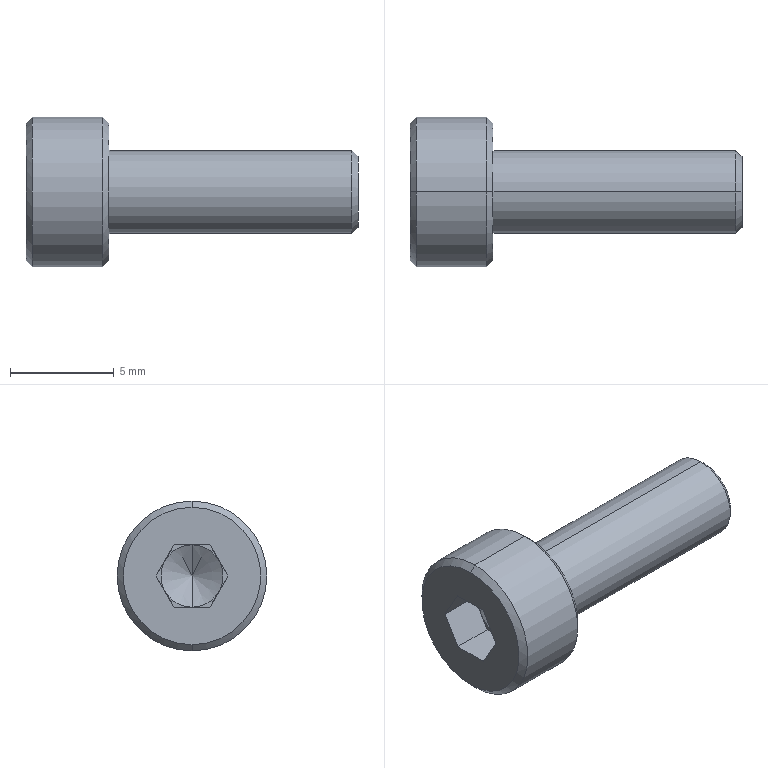Part | STEP file | Hex socket screw Dongming full thread M4-12 A2-70-1 | 1 solid | 27 faces | box 16 x 7.22 x 7.22 mm | volume 294.412 mm3 | plane 15 | cone 8 | cylinder 4 | commonest cylinder face diameters 4 x2 7.22 x2
STEP:
#1=CARTESIAN_POINT('',(16.,0.,-1.7));
#2=VERTEX_POINT('',#1);
#3=CARTESIAN_POINT('',(16.,0.,1.7));
#4=VERTEX_POINT('',#3);
#5=CARTESIAN_POINT('',(16.,0.,0.));
#6=DIRECTION('',(1.,0.,0.));
#7=DIRECTION('',(0.,0.,-1.));
#8=AXIS2_PLACEMENT_3D('',#5,#6,#7);
#9=CIRCLE('',#8,1.7);
#10=EDGE_CURVE('',#2,#4,#9,.T.);
#11=ORIENTED_EDGE('',*,*,#10,.F.);
#12=CARTESIAN_POINT('',(15.7,0.,-2.));
#13=VERTEX_POINT('',#12);
#14=CARTESIAN_POINT('',(16.,0.,-1.7));
#15=DIRECTION('',(-0.7071,0.,-0.7071));
#16=VECTOR('',#15,1000.);
#17=LINE('',#14,#16);
#18=EDGE_CURVE('',#2,#13,#17,.T.);
#19=ORIENTED_EDGE('',*,*,#18,.T.);
#20=CARTESIAN_POINT('',(15.7,0.,2.));
#21=VERTEX_POINT('',#20);
#22=CARTESIAN_POINT('',(15.7,0.,0.));
#23=DIRECTION('',(-1.,0.,0.));
#24=DIRECTION('',(0.,0.,-1.));
#25=AXIS2_PLACEMENT_3D('',#22,#23,#24);
#26=CIRCLE('',#25,2.);
#27=EDGE_CURVE('',#21,#13,#26,.T.);
#28=ORIENTED_EDGE('',*,*,#27,.F.);
#29=CARTESIAN_POINT('',(16.,0.,1.7));
#30=DIRECTION('',(-0.7071,0.,0.7071));
#31=VECTOR('',#30,1000.);
#32=LINE('',#29,#31);
#33=EDGE_CURVE('',#4,#21,#32,.T.);
#34=ORIENTED_EDGE('',*,*,#33,.F.);
#35=EDGE_LOOP('',(#11,#19,#28,#34));
#36=FACE_OUTER_BOUND('',#35,.T.);
#37=CARTESIAN_POINT('',(16.,0.,0.));
#38=DIRECTION('',(-1.,0.,0.));
#39=DIRECTION('',(0.,0.,1.));
#40=AXIS2_PLACEMENT_3D('',#37,#38,#39);
#41=CONICAL_SURFACE('',#40,1.7,0.7854);
#42=ADVANCED_FACE('',(#36),#41,.T.);
#43=CARTESIAN_POINT('',(4.,0.,-3.31));
#44=VERTEX_POINT('',#43);
#45=CARTESIAN_POINT('',(4.,0.,3.31));
#46=VERTEX_POINT('',#45);
#47=CARTESIAN_POINT('',(4.,0.,0.));
#48=DIRECTION('',(1.,0.,0.));
#49=DIRECTION('',(0.,0.,-1.));
#50=AXIS2_PLACEMENT_3D('',#47,#48,#49);
#51=CIRCLE('',#50,3.31);
#52=EDGE_CURVE('',#44,#46,#51,.T.);
#53=ORIENTED_EDGE('',*,*,#52,.F.);
#54=CARTESIAN_POINT('',(3.7,0.,-3.61));
#55=VERTEX_POINT('',#54);
#56=CARTESIAN_POINT('',(4.,0.,-3.31));
#57=DIRECTION('',(-0.7071,0.,-0.7071));
#58=VECTOR('',#57,1000.);
#59=LINE('',#56,#58);
#60=EDGE_CURVE('',#44,#55,#59,.T.);
#61=ORIENTED_EDGE('',*,*,#60,.T.);
#62=CARTESIAN_POINT('',(3.7,0.,3.61));
#63=VERTEX_POINT('',#62);
#64=CARTESIAN_POINT('',(3.7,0.,0.));
#65=DIRECTION('',(-1.,0.,0.));
#66=DIRECTION('',(0.,0.,-1.));
#67=AXIS2_PLACEMENT_3D('',#64,#65,#66);
#68=CIRCLE('',#67,3.61);
#69=EDGE_CURVE('',#63,#55,#68,.T.);
#70=ORIENTED_EDGE('',*,*,#69,.F.);
#71=CARTESIAN_POINT('',(4.,0.,3.31));
#72=DIRECTION('',(-0.7071,0.,0.7071));
#73=VECTOR('',#72,1000.);
#74=LINE('',#71,#73);
#75=EDGE_CURVE('',#46,#63,#74,.T.);
#76=ORIENTED_EDGE('',*,*,#75,.F.);
#77=EDGE_LOOP('',(#53,#61,#70,#76));
#78=FACE_OUTER_BOUND('',#77,.T.);
#79=CARTESIAN_POINT('',(4.,0.,0.));
#80=DIRECTION('',(-1.,0.,0.));
#81=DIRECTION('',(0.,0.,1.));
#82=AXIS2_PLACEMENT_3D('',#79,#80,#81);
#83=CONICAL_SURFACE('',#82,3.31,0.7854);
#84=ADVANCED_FACE('',(#78),#83,.T.);
#85=CARTESIAN_POINT('',(0.,0.,3.31));
#86=VERTEX_POINT('',#85);
#87=CARTESIAN_POINT('',(0.,0.,-3.31));
#88=VERTEX_POINT('',#87);
#89=CARTESIAN_POINT('',(0.,0.,0.));
#90=DIRECTION('',(-1.,0.,0.));
#91=DIRECTION('',(0.,0.,-1.));
#92=AXIS2_PLACEMENT_3D('',#89,#90,#91);
#93=CIRCLE('',#92,3.31);
#94=EDGE_CURVE('',#86,#88,#93,.T.);
#95=ORIENTED_EDGE('',*,*,#94,.F.);
#96=CARTESIAN_POINT('',(0.3,0.,3.61));
#97=VERTEX_POINT('',#96);
#98=CARTESIAN_POINT('',(0.3,0.,3.61));
#99=DIRECTION('',(0.7071,0.,0.7071));
#100=VECTOR('',#99,1000.);
#101=LINE('',#98,#100);
#102=EDGE_CURVE('',#86,#97,#101,.T.);
#103=ORIENTED_EDGE('',*,*,#102,.T.);
#104=CARTESIAN_POINT('',(0.3,0.,-3.61));
#105=VERTEX_POINT('',#104);
#106=CARTESIAN_POINT('',(0.3,0.,0.));
#107=DIRECTION('',(1.,0.,0.));
#108=DIRECTION('',(0.,0.,-1.));
#109=AXIS2_PLACEMENT_3D('',#106,#107,#108);
#110=CIRCLE('',#109,3.61);
#111=EDGE_CURVE('',#105,#97,#110,.T.);
#112=ORIENTED_EDGE('',*,*,#111,.F.);
#113=CARTESIAN_POINT('',(0.3,0.,-3.61));
#114=DIRECTION('',(0.7071,0.,-0.7071));
#115=VECTOR('',#114,1000.);
#116=LINE('',#113,#115);
#117=EDGE_CURVE('',#88,#105,#116,.T.);
#118=ORIENTED_EDGE('',*,*,#117,.F.);
#119=EDGE_LOOP('',(#95,#103,#112,#118));
#120=FACE_OUTER_BOUND('',#119,.T.);
#121=CARTESIAN_POINT('',(0.3,0.,0.));
#122=DIRECTION('',(1.,0.,0.));
#123=DIRECTION('',(0.,0.,-1.));
#124=AXIS2_PLACEMENT_3D('',#121,#122,#123);
#125=CONICAL_SURFACE('',#124,3.61,0.7854);
#126=ADVANCED_FACE('',(#120),#125,.T.);
#127=CARTESIAN_POINT('',(2.866,0.,0.));
#128=VERTEX_POINT('',#127);
#129=CARTESIAN_POINT('',(2.,0.,1.5));
#130=VERTEX_POINT('',#129);
#131=CARTESIAN_POINT('',(2.866,0.,0.));
#132=DIRECTION('',(-0.5,0.,0.866));
#133=VECTOR('',#132,1000.);
#134=LINE('',#131,#133);
#135=EDGE_CURVE('',#128,#130,#134,.T.);
#136=ORIENTED_EDGE('',*,*,#135,.F.);
#137=CARTESIAN_POINT('',(2.,0.,-1.5));
#138=VERTEX_POINT('',#137);
#139=CARTESIAN_POINT('',(2.866,0.,0.));
#140=DIRECTION('',(-0.5,0.,-0.866));
#141=VECTOR('',#140,1000.);
#142=LINE('',#139,#141);
#143=EDGE_CURVE('',#128,#138,#142,.T.);
#144=ORIENTED_EDGE('',*,*,#143,.T.);
#145=CARTESIAN_POINT('',(2.,-1.299,-0.75));
#146=VERTEX_POINT('',#145);
#147=CARTESIAN_POINT('',(2.,0.,0.));
#148=DIRECTION('',(-1.,0.,0.));
#149=DIRECTION('',(0.,0.,1.));
#150=AXIS2_PLACEMENT_3D('',#147,#148,#149);
#151=CIRCLE('',#150,1.5);
#152=EDGE_CURVE('',#138,#146,#151,.T.);
#153=ORIENTED_EDGE('',*,*,#152,.T.);
#154=CARTESIAN_POINT('',(2.,-1.299,0.75));
#155=VERTEX_POINT('',#154);
#156=CARTESIAN_POINT('',(2.,0.,0.));
#157=DIRECTION('',(-1.,0.,0.));
#158=DIRECTION('',(0.,0.,1.));
#159=AXIS2_PLACEMENT_3D('',#156,#157,#158);
#160=CIRCLE('',#159,1.5);
#161=EDGE_CURVE('',#146,#155,#160,.T.);
#162=ORIENTED_EDGE('',*,*,#161,.T.);
#163=CARTESIAN_POINT('',(2.,0.,0.));
#164=DIRECTION('',(-1.,0.,0.));
#165=DIRECTION('',(0.,0.,1.));
#166=AXIS2_PLACEMENT_3D('',#163,#164,#165);
#167=CIRCLE('',#166,1.5);
#168=EDGE_CURVE('',#155,#130,#167,.T.);
#169=ORIENTED_EDGE('',*,*,#168,.T.);
#170=EDGE_LOOP('',(#136,#144,#153,#162,#169));
#171=FACE_OUTER_BOUND('',#170,.T.);
#172=CARTESIAN_POINT('',(-997.134,0.,0.));
#173=DIRECTION('',(-1.,0.,0.));
#174=DIRECTION('',(0.,0.,1.));
#175=AXIS2_PLACEMENT_3D('',#172,#173,#174);
#176=CONICAL_SURFACE('',#175,1732.051,1.047);
#177=ADVANCED_FACE('',(#171),#176,.F.);
#178=ORIENTED_EDGE('',*,*,#27,.T.);
#179=CARTESIAN_POINT('',(4.,0.,-2.));
#180=VERTEX_POINT('',#179);
#181=CARTESIAN_POINT('',(16.,0.,-2.));
#182=DIRECTION('',(-1.,0.,0.));
#183=VECTOR('',#182,1000.);
#184=LINE('',#181,#183);
#185=EDGE_CURVE('',#13,#180,#184,.T.);
#186=ORIENTED_EDGE('',*,*,#185,.T.);
#187=CARTESIAN_POINT('',(4.,0.,2.));
#188=VERTEX_POINT('',#187);
#189=CARTESIAN_POINT('',(4.,0.,0.));
#190=DIRECTION('',(1.,0.,0.));
#191=DIRECTION('',(0.,0.,-1.));
#192=AXIS2_PLACEMENT_3D('',#189,#190,#191);
#193=CIRCLE('',#192,2.);
#194=EDGE_CURVE('',#180,#188,#193,.T.);
#195=ORIENTED_EDGE('',*,*,#194,.T.);
#196=CARTESIAN_POINT('',(16.,0.,2.));
#197=DIRECTION('',(-1.,0.,0.));
#198=VECTOR('',#197,1000.);
#199=LINE('',#196,#198);
#200=EDGE_CURVE('',#21,#188,#199,.T.);
#201=ORIENTED_EDGE('',*,*,#200,.F.);
#202=EDGE_LOOP('',(#178,#186,#195,#201));
#203=FACE_OUTER_BOUND('',#202,.T.);
#204=CARTESIAN_POINT('',(16.,0.,0.));
#205=DIRECTION('',(-1.,0.,0.));
#206=DIRECTION('',(0.,0.,1.));
#207=AXIS2_PLACEMENT_3D('',#204,#205,#206);
#208=CYLINDRICAL_SURFACE('',#207,2.);
#209=ADVANCED_FACE('',(#203),#208,.T.);
#210=ORIENTED_EDGE('',*,*,#69,.T.);
#211=CARTESIAN_POINT('',(4.,0.,-3.61));
#212=DIRECTION('',(-1.,0.,0.));
#213=VECTOR('',#212,1000.);
#214=LINE('',#211,#213);
#215=EDGE_CURVE('',#55,#105,#214,.T.);
#216=ORIENTED_EDGE('',*,*,#215,.T.);
#217=ORIENTED_EDGE('',*,*,#111,.T.);
#218=CARTESIAN_POINT('',(4.,0.,3.61));
#219=DIRECTION('',(-1.,0.,0.));
#220=VECTOR('',#219,1000.);
#221=LINE('',#218,#220);
#222=EDGE_CURVE('',#63,#97,#221,.T.);
#223=ORIENTED_EDGE('',*,*,#222,.F.);
#224=EDGE_LOOP('',(#210,#216,#217,#223));
#225=FACE_OUTER_BOUND('',#224,.T.);
#226=CARTESIAN_POINT('',(4.,0.,0.));
#227=DIRECTION('',(-1.,0.,0.));
#228=DIRECTION('',(0.,0.,1.));
#229=AXIS2_PLACEMENT_3D('',#226,#227,#228);
#230=CYLINDRICAL_SURFACE('',#229,3.61);
#231=ADVANCED_FACE('',(#225),#230,.T.);
#232=CARTESIAN_POINT('',(2.,1.299,0.75));
#233=VERTEX_POINT('',#232);
#234=CARTESIAN_POINT('',(2.,0.,0.));
#235=DIRECTION('',(-1.,0.,0.));
#236=DIRECTION('',(0.,0.,1.));
#237=AXIS2_PLACEMENT_3D('',#234,#235,#236);
#238=CIRCLE('',#237,1.5);
#239=EDGE_CURVE('',#130,#233,#238,.T.);
#240=ORIENTED_EDGE('',*,*,#239,.F.);
#241=CARTESIAN_POINT('',(2.,0.866,1.5));
#242=VERTEX_POINT('',#241);
#243=CARTESIAN_POINT('',(2.,-0.866,1.5));
#244=DIRECTION('',(0.,1.,0.));
#245=VECTOR('',#244,1000.);
#246=LINE('',#243,#245);
#247=EDGE_CURVE('',#130,#242,#246,.T.);
#248=ORIENTED_EDGE('',*,*,#247,.T.);
#249=CARTESIAN_POINT('',(2.,0.866,1.5));
#250=DIRECTION('',(0.,0.5,-0.866));
#251=VECTOR('',#250,1000.);
#252=LINE('',#249,#251);
#253=EDGE_CURVE('',#242,#233,#252,.T.);
#254=ORIENTED_EDGE('',*,*,#253,.T.);
#255=EDGE_LOOP('',(#240,#248,#254));
#256=FACE_OUTER_BOUND('',#255,.T.);
#257=CARTESIAN_POINT('',(2.,0.,0.));
#258=DIRECTION('',(-1.,0.,0.));
#259=DIRECTION('',(0.,0.,1.));
#260=AXIS2_PLACEMENT_3D('',#257,#258,#259);
#261=PLANE('',#260);
#262=ADVANCED_FACE('',(#256),#261,.T.);
#263=CARTESIAN_POINT('',(2.,1.299,-0.75));
#264=VERTEX_POINT('',#263);
#265=CARTESIAN_POINT('',(2.,0.,0.));
#266=DIRECTION('',(-1.,0.,0.));
#267=DIRECTION('',(0.,0.,1.));
#268=AXIS2_PLACEMENT_3D('',#265,#266,#267);
#269=CIRCLE('',#268,1.5);
#270=EDGE_CURVE('',#233,#264,#269,.T.);
#271=ORIENTED_EDGE('',*,*,#270,.F.);
#272=CARTESIAN_POINT('',(2.,1.732,0.));
#273=VERTEX_POINT('',#272);
#274=CARTESIAN_POINT('',(2.,0.866,1.5));
#275=DIRECTION('',(0.,0.5,-0.866));
#276=VECTOR('',#275,1000.);
#277=LINE('',#274,#276);
#278=EDGE_CURVE('',#233,#273,#277,.T.);
#279=ORIENTED_EDGE('',*,*,#278,.T.);
#280=CARTESIAN_POINT('',(2.,1.732,0.));
#281=DIRECTION('',(0.,-0.5,-0.866));
#282=VECTOR('',#281,1000.);
#283=LINE('',#280,#282);
#284=EDGE_CURVE('',#273,#264,#283,.T.);
#285=ORIENTED_EDGE('',*,*,#284,.T.);
#286=EDGE_LOOP('',(#271,#279,#285));
#287=FACE_OUTER_BOUND('',#286,.T.);
#288=CARTESIAN_POINT('',(2.,0.,0.));
#289=DIRECTION('',(-1.,0.,0.));
#290=DIRECTION('',(0.,0.,1.));
#291=AXIS2_PLACEMENT_3D('',#288,#289,#290);
#292=PLANE('',#291);
#293=ADVANCED_FACE('',(#287),#292,.T.);
#294=CARTESIAN_POINT('',(2.,0.,0.));
#295=DIRECTION('',(-1.,0.,0.));
#296=DIRECTION('',(0.,0.,1.));
#297=AXIS2_PLACEMENT_3D('',#294,#295,#296);
#298=CIRCLE('',#297,1.5);
#299=EDGE_CURVE('',#264,#138,#298,.T.);
#300=ORIENTED_EDGE('',*,*,#299,.F.);
#301=CARTESIAN_POINT('',(2.,0.866,-1.5));
#302=VERTEX_POINT('',#301);
#303=CARTESIAN_POINT('',(2.,1.732,0.));
#304=DIRECTION('',(0.,-0.5,-0.866));
#305=VECTOR('',#304,1000.);
#306=LINE('',#303,#305);
#307=EDGE_CURVE('',#264,#302,#306,.T.);
#308=ORIENTED_EDGE('',*,*,#307,.T.);
#309=CARTESIAN_POINT('',(2.,0.866,-1.5));
#310=DIRECTION('',(0.,-1.,0.));
#311=VECTOR('',#310,1000.);
#312=LINE('',#309,#311);
#313=EDGE_CURVE('',#302,#138,#312,.T.);
#314=ORIENTED_EDGE('',*,*,#313,.T.);
#315=EDGE_LOOP('',(#300,#308,#314));
#316=FACE_OUTER_BOUND('',#315,.T.);
#317=CARTESIAN_POINT('',(2.,0.,0.));
#318=DIRECTION('',(-1.,0.,0.));
#319=DIRECTION('',(0.,0.,1.));
#320=AXIS2_PLACEMENT_3D('',#317,#318,#319);
#321=PLANE('',#320);
#322=ADVANCED_FACE('',(#316),#321,.T.);
#323=ORIENTED_EDGE('',*,*,#152,.F.);
#324=CARTESIAN_POINT('',(2.,-0.866,-1.5));
#325=VERTEX_POINT('',#324);
#326=CARTESIAN_POINT('',(2.,0.866,-1.5));
#327=DIRECTION('',(0.,-1.,0.));
#328=VECTOR('',#327,1000.);
#329=LINE('',#326,#328);
#330=EDGE_CURVE('',#138,#325,#329,.T.);
#331=ORIENTED_EDGE('',*,*,#330,.T.);
#332=CARTESIAN_POINT('',(2.,-0.866,-1.5));
#333=DIRECTION('',(0.,-0.5,0.866));
#334=VECTOR('',#333,1000.);
#335=LINE('',#332,#334);
#336=EDGE_CURVE('',#325,#146,#335,.T.);
#337=ORIENTED_EDGE('',*,*,#336,.T.);
#338=EDGE_LOOP('',(#323,#331,#337));
#339=FACE_OUTER_BOUND('',#338,.T.);
#340=CARTESIAN_POINT('',(2.,0.,0.));
#341=DIRECTION('',(-1.,0.,0.));
#342=DIRECTION('',(0.,0.,1.));
#343=AXIS2_PLACEMENT_3D('',#340,#341,#342);
#344=PLANE('',#343);
#345=ADVANCED_FACE('',(#339),#344,.T.);
#346=ORIENTED_EDGE('',*,*,#161,.F.);
#347=CARTESIAN_POINT('',(2.,-1.732,0.));
#348=VERTEX_POINT('',#347);
#349=CARTESIAN_POINT('',(2.,-0.866,-1.5));
#350=DIRECTION('',(0.,-0.5,0.866));
#351=VECTOR('',#350,1000.);
#352=LINE('',#349,#351);
#353=EDGE_CURVE('',#146,#348,#352,.T.);
#354=ORIENTED_EDGE('',*,*,#353,.T.);
#355=CARTESIAN_POINT('',(2.,-1.732,0.));
#356=DIRECTION('',(0.,0.5,0.866));
#357=VECTOR('',#356,1000.);
#358=LINE('',#355,#357);
#359=EDGE_CURVE('',#348,#155,#358,.T.);
#360=ORIENTED_EDGE('',*,*,#359,.T.);
#361=EDGE_LOOP('',(#346,#354,#360));
#362=FACE_OUTER_BOUND('',#361,.T.);
#363=CARTESIAN_POINT('',(2.,0.,0.));
#364=DIRECTION('',(-1.,0.,0.));
#365=DIRECTION('',(0.,0.,1.));
#366=AXIS2_PLACEMENT_3D('',#363,#364,#365);
#367=PLANE('',#366);
#368=ADVANCED_FACE('',(#362),#367,.T.);
#369=ORIENTED_EDGE('',*,*,#215,.F.);
#370=CARTESIAN_POINT('',(3.7,0.,0.));
#371=DIRECTION('',(-1.,0.,0.));
#372=DIRECTION('',(0.,0.,-1.));
#373=AXIS2_PLACEMENT_3D('',#370,#371,#372);
#374=CIRCLE('',#373,3.61);
#375=EDGE_CURVE('',#55,#63,#374,.T.);
#376=ORIENTED_EDGE('',*,*,#375,.T.);
#377=ORIENTED_EDGE('',*,*,#222,.T.);
#378=CARTESIAN_POINT('',(0.3,0.,0.));
#379=DIRECTION('',(1.,0.,0.));
#380=DIRECTION('',(0.,0.,-1.));
#381=AXIS2_PLACEMENT_3D('',#378,#379,#380);
#382=CIRCLE('',#381,3.61);
#383=EDGE_CURVE('',#97,#105,#382,.T.);
#384=ORIENTED_EDGE('',*,*,#383,.T.);
#385=EDGE_LOOP('',(#369,#376,#377,#384));
#386=FACE_OUTER_BOUND('',#385,.T.);
#387=CARTESIAN_POINT('',(4.,0.,0.));
#388=DIRECTION('',(-1.,0.,0.));
#389=DIRECTION('',(0.,0.,1.));
#390=AXIS2_PLACEMENT_3D('',#387,#388,#389);
#391=CYLINDRICAL_SURFACE('',#390,3.61);
#392=ADVANCED_FACE('',(#386),#391,.T.);
#393=CARTESIAN_POINT('',(4.,0.,0.));
#394=DIRECTION('',(1.,0.,0.));
#395=DIRECTION('',(0.,0.,-1.));
#396=AXIS2_PLACEMENT_3D('',#393,#394,#395);
#397=CIRCLE('',#396,3.31);
#398=EDGE_CURVE('',#46,#44,#397,.T.);
#399=ORIENTED_EDGE('',*,*,#398,.T.);
#400=ORIENTED_EDGE('',*,*,#52,.T.);
#401=EDGE_LOOP('',(#399,#400));
#402=FACE_OUTER_BOUND('',#401,.T.);
#403=CARTESIAN_POINT('',(4.,0.,0.));
#404=DIRECTION('',(1.,0.,0.));
#405=DIRECTION('',(0.,0.,-1.));
#406=AXIS2_PLACEMENT_3D('',#403,#404,#405);
#407=CIRCLE('',#406,2.);
#408=EDGE_CURVE('',#188,#180,#407,.T.);
#409=ORIENTED_EDGE('',*,*,#408,.F.);
#410=ORIENTED_EDGE('',*,*,#194,.F.);
#411=EDGE_LOOP('',(#409,#410));
#412=FACE_BOUND('',#411,.T.);
#413=CARTESIAN_POINT('',(4.,0.,0.));
#414=DIRECTION('',(1.,0.,0.));
#415=DIRECTION('',(0.,0.,-1.));
#416=AXIS2_PLACEMENT_3D('',#413,#414,#415);
#417=PLANE('',#416);
#418=ADVANCED_FACE('',(#402,#412),#417,.T.);
#419=CARTESIAN_POINT('',(0.,0.,0.));
#420=DIRECTION('',(-1.,0.,0.));
#421=DIRECTION('',(0.,0.,-1.));
#422=AXIS2_PLACEMENT_3D('',#419,#420,#421);
#423=CIRCLE('',#422,3.31);
#424=EDGE_CURVE('',#88,#86,#423,.T.);
#425=ORIENTED_EDGE('',*,*,#424,.T.);
#426=ORIENTED_EDGE('',*,*,#94,.T.);
#427=EDGE_LOOP('',(#425,#426));
#428=FACE_OUTER_BOUND('',#427,.T.);
#429=CARTESIAN_POINT('',(0.,1.732,0.));
#430=VERTEX_POINT('',#429);
#431=CARTESIAN_POINT('',(0.,0.866,-1.5));
#432=VERTEX_POINT('',#431);
#433=CARTESIAN_POINT('',(0.,1.732,0.));
#434=DIRECTION('',(0.,-0.5,-0.866));
#435=VECTOR('',#434,1000.);
#436=LINE('',#433,#435);
#437=EDGE_CURVE('',#430,#432,#436,.T.);
#438=ORIENTED_EDGE('',*,*,#437,.F.);
#439=CARTESIAN_POINT('',(0.,0.866,1.5));
#440=VERTEX_POINT('',#439);
#441=CARTESIAN_POINT('',(0.,0.866,1.5));
#442=DIRECTION('',(0.,0.5,-0.866));
#443=VECTOR('',#442,1000.);
#444=LINE('',#441,#443);
#445=EDGE_CURVE('',#440,#430,#444,.T.);
#446=ORIENTED_EDGE('',*,*,#445,.F.);
#447=CARTESIAN_POINT('',(0.,-0.866,1.5));
#448=VERTEX_POINT('',#447);
#449=CARTESIAN_POINT('',(0.,-0.866,1.5));
#450=DIRECTION('',(0.,1.,0.));
#451=VECTOR('',#450,1000.);
#452=LINE('',#449,#451);
#453=EDGE_CURVE('',#448,#440,#452,.T.);
#454=ORIENTED_EDGE('',*,*,#453,.F.);
#455=CARTESIAN_POINT('',(0.,-1.732,0.));
#456=VERTEX_POINT('',#455);
#457=CARTESIAN_POINT('',(0.,-1.732,0.));
#458=DIRECTION('',(0.,0.5,0.866));
#459=VECTOR('',#458,1000.);
#460=LINE('',#457,#459);
#461=EDGE_CURVE('',#456,#448,#460,.T.);
#462=ORIENTED_EDGE('',*,*,#461,.F.);
#463=CARTESIAN_POINT('',(0.,-0.866,-1.5));
#464=VERTEX_POINT('',#463);
#465=CARTESIAN_POINT('',(0.,-0.866,-1.5));
#466=DIRECTION('',(0.,-0.5,0.866));
#467=VECTOR('',#466,1000.);
#468=LINE('',#465,#467);
#469=EDGE_CURVE('',#464,#456,#468,.T.);
#470=ORIENTED_EDGE('',*,*,#469,.F.);
#471=CARTESIAN_POINT('',(0.,0.866,-1.5));
#472=DIRECTION('',(0.,-1.,0.));
#473=VECTOR('',#472,1000.);
#474=LINE('',#471,#473);
#475=EDGE_CURVE('',#432,#464,#474,.T.);
#476=ORIENTED_EDGE('',*,*,#475,.F.);
#477=EDGE_LOOP('',(#438,#446,#454,#462,#470,#476));
#478=FACE_BOUND('',#477,.T.);
#479=CARTESIAN_POINT('',(0.,0.,0.));
#480=DIRECTION('',(1.,0.,0.));
#481=DIRECTION('',(0.,0.,-1.));
#482=AXIS2_PLACEMENT_3D('',#479,#480,#481);
#483=PLANE('',#482);
#484=ADVANCED_FACE('',(#428,#478),#483,.F.);
#485=ORIENTED_EDGE('',*,*,#185,.F.);
#486=CARTESIAN_POINT('',(15.7,0.,0.));
#487=DIRECTION('',(-1.,0.,0.));
#488=DIRECTION('',(0.,0.,-1.));
#489=AXIS2_PLACEMENT_3D('',#486,#487,#488);
#490=CIRCLE('',#489,2.);
#491=EDGE_CURVE('',#13,#21,#490,.T.);
#492=ORIENTED_EDGE('',*,*,#491,.T.);
#493=ORIENTED_EDGE('',*,*,#200,.T.);
#494=ORIENTED_EDGE('',*,*,#408,.T.);
#495=EDGE_LOOP('',(#485,#492,#493,#494));
#496=FACE_OUTER_BOUND('',#495,.T.);
#497=CARTESIAN_POINT('',(16.,0.,0.));
#498=DIRECTION('',(-1.,0.,0.));
#499=DIRECTION('',(0.,0.,1.));
#500=AXIS2_PLACEMENT_3D('',#497,#498,#499);
#501=CYLINDRICAL_SURFACE('',#500,2.);
#502=ADVANCED_FACE('',(#496),#501,.T.);
#503=CARTESIAN_POINT('',(16.,0.,0.));
#504=DIRECTION('',(1.,0.,0.));
#505=DIRECTION('',(0.,0.,-1.));
#506=AXIS2_PLACEMENT_3D('',#503,#504,#505);
#507=CIRCLE('',#506,1.7);
#508=EDGE_CURVE('',#4,#2,#507,.T.);
#509=ORIENTED_EDGE('',*,*,#508,.T.);
#510=ORIENTED_EDGE('',*,*,#10,.T.);
#511=EDGE_LOOP('',(#509,#510));
#512=FACE_OUTER_BOUND('',#511,.T.);
#513=CARTESIAN_POINT('',(16.,0.,0.));
#514=DIRECTION('',(1.,0.,0.));
#515=DIRECTION('',(0.,0.,-1.));
#516=AXIS2_PLACEMENT_3D('',#513,#514,#515);
#517=PLANE('',#516);
#518=ADVANCED_FACE('',(#512),#517,.T.);
#519=ORIENTED_EDGE('',*,*,#445,.T.);
#520=CARTESIAN_POINT('',(2.,1.732,0.));
#521=DIRECTION('',(-1.,0.,0.));
#522=VECTOR('',#521,1000.);
#523=LINE('',#520,#522);
#524=EDGE_CURVE('',#273,#430,#523,.T.);
#525=ORIENTED_EDGE('',*,*,#524,.F.);
#526=ORIENTED_EDGE('',*,*,#278,.F.);
#527=ORIENTED_EDGE('',*,*,#253,.F.);
#528=CARTESIAN_POINT('',(2.,0.866,1.5));
#529=DIRECTION('',(-1.,0.,0.));
#530=VECTOR('',#529,1000.);
#531=LINE('',#528,#530);
#532=EDGE_CURVE('',#242,#440,#531,.T.);
#533=ORIENTED_EDGE('',*,*,#532,.T.);
#534=EDGE_LOOP('',(#519,#525,#526,#527,#533));
#535=FACE_OUTER_BOUND('',#534,.T.);
#536=CARTESIAN_POINT('',(2.,0.866,1.5));
#537=DIRECTION('',(0.,0.866,0.5));
#538=DIRECTION('',(0.,-0.5,0.866));
#539=AXIS2_PLACEMENT_3D('',#536,#537,#538);
#540=PLANE('',#539);
#541=ADVANCED_FACE('',(#535),#540,.F.);
#542=ORIENTED_EDGE('',*,*,#453,.T.);
#543=ORIENTED_EDGE('',*,*,#532,.F.);
#544=ORIENTED_EDGE('',*,*,#247,.F.);
#545=CARTESIAN_POINT('',(2.,-0.866,1.5));
#546=VERTEX_POINT('',#545);
#547=CARTESIAN_POINT('',(2.,-0.866,1.5));
#548=DIRECTION('',(0.,1.,0.));
#549=VECTOR('',#548,1000.);
#550=LINE('',#547,#549);
#551=EDGE_CURVE('',#546,#130,#550,.T.);
#552=ORIENTED_EDGE('',*,*,#551,.F.);
#553=CARTESIAN_POINT('',(2.,-0.866,1.5));
#554=DIRECTION('',(-1.,0.,0.));
#555=VECTOR('',#554,1000.);
#556=LINE('',#553,#555);
#557=EDGE_CURVE('',#546,#448,#556,.T.);
#558=ORIENTED_EDGE('',*,*,#557,.T.);
#559=EDGE_LOOP('',(#542,#543,#544,#552,#558));
#560=FACE_OUTER_BOUND('',#559,.T.);
#561=CARTESIAN_POINT('',(2.,-0.866,1.5));
#562=DIRECTION('',(0.,0.,1.));
#563=DIRECTION('',(0.,-1.,0.));
#564=AXIS2_PLACEMENT_3D('',#561,#562,#563);
#565=PLANE('',#564);
#566=ADVANCED_FACE('',(#560),#565,.F.);
#567=ORIENTED_EDGE('',*,*,#461,.T.);
#568=ORIENTED_EDGE('',*,*,#557,.F.);
#569=CARTESIAN_POINT('',(2.,-1.732,0.));
#570=DIRECTION('',(0.,0.5,0.866));
#571=VECTOR('',#570,1000.);
#572=LINE('',#569,#571);
#573=EDGE_CURVE('',#155,#546,#572,.T.);
#574=ORIENTED_EDGE('',*,*,#573,.F.);
#575=ORIENTED_EDGE('',*,*,#359,.F.);
#576=CARTESIAN_POINT('',(2.,-1.732,0.));
#577=DIRECTION('',(-1.,0.,0.));
#578=VECTOR('',#577,1000.);
#579=LINE('',#576,#578);
#580=EDGE_CURVE('',#348,#456,#579,.T.);
#581=ORIENTED_EDGE('',*,*,#580,.T.);
#582=EDGE_LOOP('',(#567,#568,#574,#575,#581));
#583=FACE_OUTER_BOUND('',#582,.T.);
#584=CARTESIAN_POINT('',(2.,-1.732,0.));
#585=DIRECTION('',(0.,-0.866,0.5));
#586=DIRECTION('',(0.,-0.5,-0.866));
#587=AXIS2_PLACEMENT_3D('',#584,#585,#586);
#588=PLANE('',#587);
#589=ADVANCED_FACE('',(#583),#588,.F.);
#590=ORIENTED_EDGE('',*,*,#469,.T.);
#591=ORIENTED_EDGE('',*,*,#580,.F.);
#592=ORIENTED_EDGE('',*,*,#353,.F.);
#593=ORIENTED_EDGE('',*,*,#336,.F.);
#594=CARTESIAN_POINT('',(2.,-0.866,-1.5));
#595=DIRECTION('',(-1.,0.,0.));
#596=VECTOR('',#595,1000.);
#597=LINE('',#594,#596);
#598=EDGE_CURVE('',#325,#464,#597,.T.);
#599=ORIENTED_EDGE('',*,*,#598,.T.);
#600=EDGE_LOOP('',(#590,#591,#592,#593,#599));
#601=FACE_OUTER_BOUND('',#600,.T.);
#602=CARTESIAN_POINT('',(2.,-0.866,-1.5));
#603=DIRECTION('',(0.,-0.866,-0.5));
#604=DIRECTION('',(0.,0.5,-0.866));
#605=AXIS2_PLACEMENT_3D('',#602,#603,#604);
#606=PLANE('',#605);
#607=ADVANCED_FACE('',(#601),#606,.F.);
#608=ORIENTED_EDGE('',*,*,#475,.T.);
#609=ORIENTED_EDGE('',*,*,#598,.F.);
#610=ORIENTED_EDGE('',*,*,#330,.F.);
#611=ORIENTED_EDGE('',*,*,#313,.F.);
#612=CARTESIAN_POINT('',(2.,0.866,-1.5));
#613=DIRECTION('',(-1.,0.,0.));
#614=VECTOR('',#613,1000.);
#615=LINE('',#612,#614);
#616=EDGE_CURVE('',#302,#432,#615,.T.);
#617=ORIENTED_EDGE('',*,*,#616,.T.);
#618=EDGE_LOOP('',(#608,#609,#610,#611,#617));
#619=FACE_OUTER_BOUND('',#618,.T.);
#620=CARTESIAN_POINT('',(2.,0.866,-1.5));
#621=DIRECTION('',(0.,0.,-1.));
#622=DIRECTION('',(-1.,0.,0.));
#623=AXIS2_PLACEMENT_3D('',#620,#621,#622);
#624=PLANE('',#623);
#625=ADVANCED_FACE('',(#619),#624,.F.);
#626=ORIENTED_EDGE('',*,*,#437,.T.);
#627=ORIENTED_EDGE('',*,*,#616,.F.);
#628=ORIENTED_EDGE('',*,*,#307,.F.);
#629=ORIENTED_EDGE('',*,*,#284,.F.);
#630=ORIENTED_EDGE('',*,*,#524,.T.);
#631=EDGE_LOOP('',(#626,#627,#628,#629,#630));
#632=FACE_OUTER_BOUND('',#631,.T.);
#633=CARTESIAN_POINT('',(2.,1.732,0.));
#634=DIRECTION('',(0.,0.866,-0.5));
#635=DIRECTION('',(0.,0.5,0.866));
#636=AXIS2_PLACEMENT_3D('',#633,#634,#635);
#637=PLANE('',#636);
#638=ADVANCED_FACE('',(#632),#637,.F.);
#639=ORIENTED_EDGE('',*,*,#168,.F.);
#640=ORIENTED_EDGE('',*,*,#573,.T.);
#641=ORIENTED_EDGE('',*,*,#551,.T.);
#642=EDGE_LOOP('',(#639,#640,#641));
#643=FACE_OUTER_BOUND('',#642,.T.);
#644=CARTESIAN_POINT('',(2.,0.,0.));
#645=DIRECTION('',(-1.,0.,0.));
#646=DIRECTION('',(0.,0.,1.));
#647=AXIS2_PLACEMENT_3D('',#644,#645,#646);
#648=PLANE('',#647);
#649=ADVANCED_FACE('',(#643),#648,.T.);
#650=ORIENTED_EDGE('',*,*,#143,.F.);
#651=ORIENTED_EDGE('',*,*,#135,.T.);
#652=ORIENTED_EDGE('',*,*,#239,.T.);
#653=ORIENTED_EDGE('',*,*,#270,.T.);
#654=ORIENTED_EDGE('',*,*,#299,.T.);
#655=EDGE_LOOP('',(#650,#651,#652,#653,#654));
#656=FACE_OUTER_BOUND('',#655,.T.);
#657=CARTESIAN_POINT('',(-997.134,0.,0.));
#658=DIRECTION('',(-1.,0.,0.));
#659=DIRECTION('',(0.,0.,1.));
#660=AXIS2_PLACEMENT_3D('',#657,#658,#659);
#661=CONICAL_SURFACE('',#660,1732.051,1.047);
#662=ADVANCED_FACE('',(#656),#661,.F.);
#663=ORIENTED_EDGE('',*,*,#102,.F.);
#664=ORIENTED_EDGE('',*,*,#424,.F.);
#665=ORIENTED_EDGE('',*,*,#117,.T.);
#666=ORIENTED_EDGE('',*,*,#383,.F.);
#667=EDGE_LOOP('',(#663,#664,#665,#666));
#668=FACE_OUTER_BOUND('',#667,.T.);
#669=CARTESIAN_POINT('',(0.3,0.,0.));
#670=DIRECTION('',(1.,0.,0.));
#671=DIRECTION('',(0.,0.,-1.));
#672=AXIS2_PLACEMENT_3D('',#669,#670,#671);
#673=CONICAL_SURFACE('',#672,3.61,0.7854);
#674=ADVANCED_FACE('',(#668),#673,.T.);
#675=ORIENTED_EDGE('',*,*,#60,.F.);
#676=ORIENTED_EDGE('',*,*,#398,.F.);
#677=ORIENTED_EDGE('',*,*,#75,.T.);
#678=ORIENTED_EDGE('',*,*,#375,.F.);
#679=EDGE_LOOP('',(#675,#676,#677,#678));
#680=FACE_OUTER_BOUND('',#679,.T.);
#681=CARTESIAN_POINT('',(4.,0.,0.));
#682=DIRECTION('',(-1.,0.,0.));
#683=DIRECTION('',(0.,0.,1.));
#684=AXIS2_PLACEMENT_3D('',#681,#682,#683);
#685=CONICAL_SURFACE('',#684,3.31,0.7854);
#686=ADVANCED_FACE('',(#680),#685,.T.);
#687=ORIENTED_EDGE('',*,*,#18,.F.);
#688=ORIENTED_EDGE('',*,*,#508,.F.);
#689=ORIENTED_EDGE('',*,*,#33,.T.);
#690=ORIENTED_EDGE('',*,*,#491,.F.);
#691=EDGE_LOOP('',(#687,#688,#689,#690));
#692=FACE_OUTER_BOUND('',#691,.T.);
#693=CARTESIAN_POINT('',(16.,0.,0.));
#694=DIRECTION('',(-1.,0.,0.));
#695=DIRECTION('',(0.,0.,1.));
#696=AXIS2_PLACEMENT_3D('',#693,#694,#695);
#697=CONICAL_SURFACE('',#696,1.7,0.7854);
#698=ADVANCED_FACE('',(#692),#697,.T.);
#699=CLOSED_SHELL('',(#42,#84,#126,#177,#209,#231,#262,#293,#322,#345,#368,#392,#418,#484,#502,#518,#541,#566,#589,#607,#625,#638,#649,#662,#674,#686,#698));
#700=MANIFOLD_SOLID_BREP('',#699);
#701=CARTESIAN_POINT('',(0.,0.,0.));
#702=DIRECTION('',(0.,0.,1.));
#703=DIRECTION('',(1.,0.,0.));
#704=AXIS2_PLACEMENT_3D('',#701,#702,#703);
#705=(LENGTH_UNIT()NAMED_UNIT(*)SI_UNIT(.MILLI.,.METRE.));
#706=UNCERTAINTY_MEASURE_WITH_UNIT(LENGTH_MEASURE(0.00001),#705,'','');
#707=(NAMED_UNIT(*)PLANE_ANGLE_UNIT()SI_UNIT($,.RADIAN.));
#708=(NAMED_UNIT(*)SI_UNIT($,.STERADIAN.)SOLID_ANGLE_UNIT());
#709=(GEOMETRIC_REPRESENTATION_CONTEXT(3)GLOBAL_UNCERTAINTY_ASSIGNED_CONTEXT((#706))GLOBAL_UNIT_ASSIGNED_CONTEXT((#705,#707,#708))REPRESENTATION_CONTEXT('',''));
#710=ADVANCED_BREP_SHAPE_REPRESENTATION('',(#700,#704),#709);